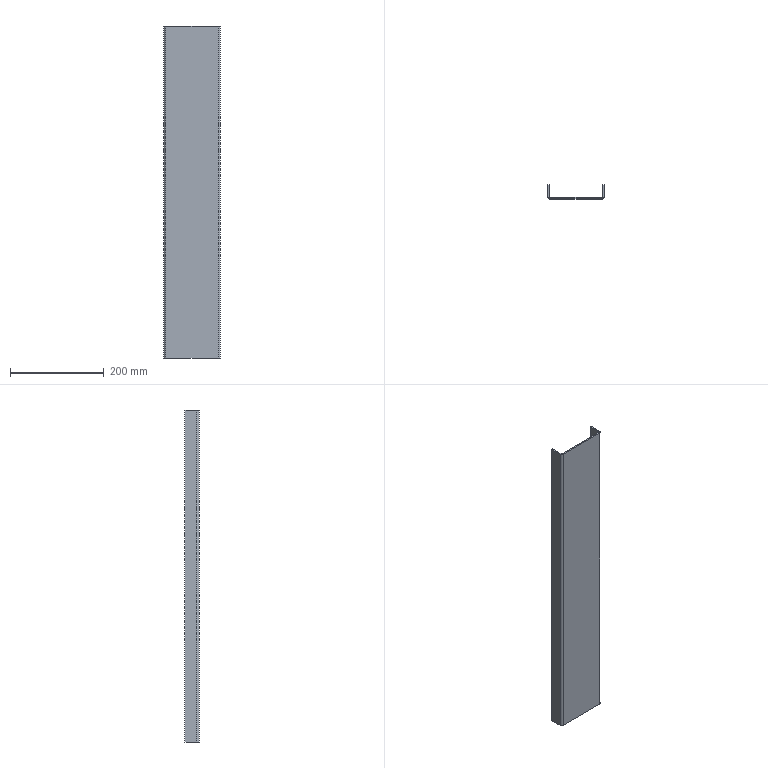Part | STEP file | Double-tube frame vertical brace SGN-1-05 | 1 solid | 22 faces | box 120 x 30 x 708 mm | volume 364106 mm3 | plane 18 | cylinder 4 | commonest cylinder face diameters 3 x2 9 x2
STEP:
#1=CARTESIAN_POINT('',(0.,0.,0.));
#2=DIRECTION('',(0.,0.,1.));
#3=DIRECTION('',(1.,0.,0.));
#4=AXIS2_PLACEMENT_3D('',#1,#2,#3);
#5=CARTESIAN_POINT('',(55.5,-6.24,708.));
#6=VERTEX_POINT('',#5);
#7=CARTESIAN_POINT('',(55.5,-3.24,708.));
#8=VERTEX_POINT('',#7);
#9=CARTESIAN_POINT('',(55.5,-6.24,708.));
#10=DIRECTION('',(0.,1.,0.));
#11=VECTOR('',#10,1.);
#12=LINE('',#9,#11);
#13=CARTESIAN_POINT('',(55.5,-6.24,708.));
#14=DIRECTION('',(0.,0.,1.));
#15=DIRECTION('',(1.,0.,0.));
#16=AXIS2_PLACEMENT_3D('',#13,#14,#15);
#17=PLANE('',#16);
#18=CARTESIAN_POINT('',(0.,0.));
#19=DIRECTION('',(0.,1.));
#20=VECTOR('',#19,1.);
#21=LINE('',#18,#20);
#22=(GEOMETRIC_REPRESENTATION_CONTEXT(2)PARAMETRIC_REPRESENTATION_CONTEXT()REPRESENTATION_CONTEXT('',''));
#23=DEFINITIONAL_REPRESENTATION('',(#21),#22);
#24=PCURVE('',#17,#23);
#25=CARTESIAN_POINT('',(57.,-1.74,708.));
#26=DIRECTION('',(0.,0.,1.));
#27=DIRECTION('',(1.,0.,0.));
#28=AXIS2_PLACEMENT_3D('',#25,#26,#27);
#29=PLANE('',#28);
#30=CARTESIAN_POINT('',(-1.5,-4.5));
#31=DIRECTION('',(0.,1.));
#32=VECTOR('',#31,1.);
#33=LINE('',#30,#32);
#34=(GEOMETRIC_REPRESENTATION_CONTEXT(2)PARAMETRIC_REPRESENTATION_CONTEXT()REPRESENTATION_CONTEXT('',''));
#35=DEFINITIONAL_REPRESENTATION('',(#33),#34);
#36=PCURVE('',#29,#35);
#37=SURFACE_CURVE('',#12,(#24,#36),.PCURVE_S1.);
#38=EDGE_CURVE('',#6,#8,#37,.T.);
#39=ORIENTED_EDGE('',*,*,#38,.F.);
#40=CARTESIAN_POINT('',(60.,-1.74,708.));
#41=VERTEX_POINT('',#40);
#42=CARTESIAN_POINT('',(55.5,-1.74,708.));
#43=DIRECTION('',(0.,0.,-1.));
#44=DIRECTION('',(1.,0.,0.));
#45=AXIS2_PLACEMENT_3D('',#42,#43,#44);
#46=CIRCLE('',#45,4.5);
#47=CARTESIAN_POINT('',(4.5,4.5));
#48=CARTESIAN_POINT('',(4.5,-3.294));
#49=CARTESIAN_POINT('',(-2.25,0.6029));
#50=CARTESIAN_POINT('',(-9.,4.5));
#51=CARTESIAN_POINT('',(-2.25,8.397));
#52=CARTESIAN_POINT('',(4.5,12.294));
#53=CARTESIAN_POINT('',(4.5,4.5));
#54=(BOUNDED_CURVE()B_SPLINE_CURVE(2,(#47,#48,#49,#50,#51,#52,#53),.UNSPECIFIED.,.T.,.F.)B_SPLINE_CURVE_WITH_KNOTS((1,2,2,2,2,1),(-2.094,0.,2.094,4.189,6.283,8.378),.UNSPECIFIED.)CURVE()GEOMETRIC_REPRESENTATION_ITEM()RATIONAL_B_SPLINE_CURVE((1.,0.5,1.,0.5,1.,0.5,1.))REPRESENTATION_ITEM(''));
#55=(GEOMETRIC_REPRESENTATION_CONTEXT(2)PARAMETRIC_REPRESENTATION_CONTEXT()REPRESENTATION_CONTEXT('',''));
#56=DEFINITIONAL_REPRESENTATION('',(#54),#55);
#57=PCURVE('',#17,#56);
#58=CARTESIAN_POINT('',(55.5,-1.74,708.));
#59=DIRECTION('',(0.,0.,-1.));
#60=DIRECTION('',(-1.,0.,0.));
#61=AXIS2_PLACEMENT_3D('',#58,#59,#60);
#62=CYLINDRICAL_SURFACE('',#61,4.5);
#63=CARTESIAN_POINT('',(3.142,0.));
#64=DIRECTION('',(1.,0.));
#65=VECTOR('',#64,1.);
#66=LINE('',#63,#65);
#67=(GEOMETRIC_REPRESENTATION_CONTEXT(2)PARAMETRIC_REPRESENTATION_CONTEXT()REPRESENTATION_CONTEXT('',''));
#68=DEFINITIONAL_REPRESENTATION('',(#66),#67);
#69=PCURVE('',#62,#68);
#70=SURFACE_CURVE('',#46,(#57,#69),.PCURVE_S1.);
#71=EDGE_CURVE('',#41,#6,#70,.T.);
#72=ORIENTED_EDGE('',*,*,#71,.F.);
#73=CARTESIAN_POINT('',(57.,-1.74,708.));
#74=VERTEX_POINT('',#73);
#75=CARTESIAN_POINT('',(57.,-1.74,708.));
#76=DIRECTION('',(1.,0.,0.));
#77=VECTOR('',#76,1.);
#78=LINE('',#75,#77);
#79=CARTESIAN_POINT('',(1.5,4.5));
#80=DIRECTION('',(1.,0.));
#81=VECTOR('',#80,1.);
#82=LINE('',#79,#81);
#83=(GEOMETRIC_REPRESENTATION_CONTEXT(2)PARAMETRIC_REPRESENTATION_CONTEXT()REPRESENTATION_CONTEXT('',''));
#84=DEFINITIONAL_REPRESENTATION('',(#82),#83);
#85=PCURVE('',#17,#84);
#86=CARTESIAN_POINT('',(-55.5,-1.74,708.));
#87=DIRECTION('',(0.,0.,1.));
#88=DIRECTION('',(1.,0.,0.));
#89=AXIS2_PLACEMENT_3D('',#86,#87,#88);
#90=PLANE('',#89);
#91=CARTESIAN_POINT('',(112.5,0.));
#92=DIRECTION('',(1.,0.));
#93=VECTOR('',#92,1.);
#94=LINE('',#91,#93);
#95=(GEOMETRIC_REPRESENTATION_CONTEXT(2)PARAMETRIC_REPRESENTATION_CONTEXT()REPRESENTATION_CONTEXT('',''));
#96=DEFINITIONAL_REPRESENTATION('',(#94),#95);
#97=PCURVE('',#90,#96);
#98=SURFACE_CURVE('',#78,(#85,#97),.PCURVE_S1.);
#99=EDGE_CURVE('',#74,#41,#98,.T.);
#100=ORIENTED_EDGE('',*,*,#99,.F.);
#101=CARTESIAN_POINT('',(55.5,-1.74,708.));
#102=DIRECTION('',(0.,0.,-1.));
#103=DIRECTION('',(1.,0.,0.));
#104=AXIS2_PLACEMENT_3D('',#101,#102,#103);
#105=CIRCLE('',#104,1.5);
#106=CARTESIAN_POINT('',(1.5,4.5));
#107=CARTESIAN_POINT('',(1.5,1.902));
#108=CARTESIAN_POINT('',(-0.75,3.201));
#109=CARTESIAN_POINT('',(-3.,4.5));
#110=CARTESIAN_POINT('',(-0.75,5.799));
#111=CARTESIAN_POINT('',(1.5,7.098));
#112=CARTESIAN_POINT('',(1.5,4.5));
#113=(BOUNDED_CURVE()B_SPLINE_CURVE(2,(#106,#107,#108,#109,#110,#111,#112),.UNSPECIFIED.,.T.,.F.)B_SPLINE_CURVE_WITH_KNOTS((1,2,2,2,2,1),(-2.094,0.,2.094,4.189,6.283,8.378),.UNSPECIFIED.)CURVE()GEOMETRIC_REPRESENTATION_ITEM()RATIONAL_B_SPLINE_CURVE((1.,0.5,1.,0.5,1.,0.5,1.))REPRESENTATION_ITEM(''));
#114=(GEOMETRIC_REPRESENTATION_CONTEXT(2)PARAMETRIC_REPRESENTATION_CONTEXT()REPRESENTATION_CONTEXT('',''));
#115=DEFINITIONAL_REPRESENTATION('',(#113),#114);
#116=PCURVE('',#17,#115);
#117=CARTESIAN_POINT('',(55.5,-1.74,708.));
#118=DIRECTION('',(0.,0.,-1.));
#119=DIRECTION('',(-1.,0.,0.));
#120=AXIS2_PLACEMENT_3D('',#117,#118,#119);
#121=CYLINDRICAL_SURFACE('',#120,1.5);
#122=CARTESIAN_POINT('',(3.142,0.));
#123=DIRECTION('',(1.,0.));
#124=VECTOR('',#123,1.);
#125=LINE('',#122,#124);
#126=(GEOMETRIC_REPRESENTATION_CONTEXT(2)PARAMETRIC_REPRESENTATION_CONTEXT()REPRESENTATION_CONTEXT('',''));
#127=DEFINITIONAL_REPRESENTATION('',(#125),#126);
#128=PCURVE('',#121,#127);
#129=SURFACE_CURVE('',#105,(#116,#128),.PCURVE_S1.);
#130=EDGE_CURVE('',#74,#8,#129,.T.);
#131=ORIENTED_EDGE('',*,*,#130,.T.);
#132=EDGE_LOOP('',(#39,#72,#100,#131));
#133=FACE_BOUND('',#132,.T.);
#134=ADVANCED_FACE('',(#133),#17,.T.);
#135=CARTESIAN_POINT('',(-55.5,-6.24,708.));
#136=VERTEX_POINT('',#135);
#137=CARTESIAN_POINT('',(-60.,-6.24,708.));
#138=DIRECTION('',(-1.,0.,0.));
#139=VECTOR('',#138,1.);
#140=LINE('',#137,#139);
#141=CARTESIAN_POINT('',(-117.,-4.5));
#142=DIRECTION('',(-1.,0.));
#143=VECTOR('',#142,1.);
#144=LINE('',#141,#143);
#145=(GEOMETRIC_REPRESENTATION_CONTEXT(2)PARAMETRIC_REPRESENTATION_CONTEXT()REPRESENTATION_CONTEXT('',''));
#146=DEFINITIONAL_REPRESENTATION('',(#144),#145);
#147=PCURVE('',#29,#146);
#148=CARTESIAN_POINT('',(-60.,-6.24,708.));
#149=DIRECTION('',(0.,-1.,0.));
#150=DIRECTION('',(0.,0.,-1.));
#151=AXIS2_PLACEMENT_3D('',#148,#149,#150);
#152=PLANE('',#151);
#153=CARTESIAN_POINT('',(0.,0.));
#154=DIRECTION('',(0.,-1.));
#155=VECTOR('',#154,1.);
#156=LINE('',#153,#155);
#157=(GEOMETRIC_REPRESENTATION_CONTEXT(2)PARAMETRIC_REPRESENTATION_CONTEXT()REPRESENTATION_CONTEXT('',''));
#158=DEFINITIONAL_REPRESENTATION('',(#156),#157);
#159=PCURVE('',#152,#158);
#160=SURFACE_CURVE('',#140,(#147,#159),.PCURVE_S1.);
#161=EDGE_CURVE('',#6,#136,#160,.T.);
#162=ORIENTED_EDGE('',*,*,#161,.F.);
#163=ORIENTED_EDGE('',*,*,#38,.T.);
#164=CARTESIAN_POINT('',(-55.5,-3.24,708.));
#165=VERTEX_POINT('',#164);
#166=CARTESIAN_POINT('',(-60.,-3.24,708.));
#167=DIRECTION('',(-1.,0.,0.));
#168=VECTOR('',#167,1.);
#169=LINE('',#166,#168);
#170=CARTESIAN_POINT('',(-117.,-1.5));
#171=DIRECTION('',(-1.,0.));
#172=VECTOR('',#171,1.);
#173=LINE('',#170,#172);
#174=(GEOMETRIC_REPRESENTATION_CONTEXT(2)PARAMETRIC_REPRESENTATION_CONTEXT()REPRESENTATION_CONTEXT('',''));
#175=DEFINITIONAL_REPRESENTATION('',(#173),#174);
#176=PCURVE('',#29,#175);
#177=CARTESIAN_POINT('',(-60.,-3.24,708.));
#178=DIRECTION('',(0.,-1.,0.));
#179=DIRECTION('',(0.,0.,-1.));
#180=AXIS2_PLACEMENT_3D('',#177,#178,#179);
#181=PLANE('',#180);
#182=CARTESIAN_POINT('',(0.,0.));
#183=DIRECTION('',(0.,-1.));
#184=VECTOR('',#183,1.);
#185=LINE('',#182,#184);
#186=(GEOMETRIC_REPRESENTATION_CONTEXT(2)PARAMETRIC_REPRESENTATION_CONTEXT()REPRESENTATION_CONTEXT('',''));
#187=DEFINITIONAL_REPRESENTATION('',(#185),#186);
#188=PCURVE('',#181,#187);
#189=SURFACE_CURVE('',#169,(#176,#188),.PCURVE_S1.);
#190=EDGE_CURVE('',#8,#165,#189,.T.);
#191=ORIENTED_EDGE('',*,*,#190,.T.);
#192=CARTESIAN_POINT('',(-55.5,-3.24,708.));
#193=DIRECTION('',(0.,-1.,0.));
#194=VECTOR('',#193,1.);
#195=LINE('',#192,#194);
#196=CARTESIAN_POINT('',(-112.5,-1.5));
#197=DIRECTION('',(0.,-1.));
#198=VECTOR('',#197,1.);
#199=LINE('',#196,#198);
#200=(GEOMETRIC_REPRESENTATION_CONTEXT(2)PARAMETRIC_REPRESENTATION_CONTEXT()REPRESENTATION_CONTEXT('',''));
#201=DEFINITIONAL_REPRESENTATION('',(#199),#200);
#202=PCURVE('',#29,#201);
#203=CARTESIAN_POINT('',(-60.,-1.74,708.));
#204=DIRECTION('',(0.,0.,1.));
#205=DIRECTION('',(1.,0.,0.));
#206=AXIS2_PLACEMENT_3D('',#203,#204,#205);
#207=PLANE('',#206);
#208=CARTESIAN_POINT('',(4.5,-1.5));
#209=DIRECTION('',(0.,-1.));
#210=VECTOR('',#209,1.);
#211=LINE('',#208,#210);
#212=(GEOMETRIC_REPRESENTATION_CONTEXT(2)PARAMETRIC_REPRESENTATION_CONTEXT()REPRESENTATION_CONTEXT('',''));
#213=DEFINITIONAL_REPRESENTATION('',(#211),#212);
#214=PCURVE('',#207,#213);
#215=SURFACE_CURVE('',#195,(#202,#214),.PCURVE_S1.);
#216=EDGE_CURVE('',#165,#136,#215,.T.);
#217=ORIENTED_EDGE('',*,*,#216,.T.);
#218=EDGE_LOOP('',(#162,#163,#191,#217));
#219=FACE_BOUND('',#218,.T.);
#220=ADVANCED_FACE('',(#219),#29,.T.);
#221=CARTESIAN_POINT('',(60.,-1.74,0.));
#222=VERTEX_POINT('',#221);
#223=CARTESIAN_POINT('',(57.,-1.74,0.));
#224=VERTEX_POINT('',#223);
#225=CARTESIAN_POINT('',(60.,-1.74,0.));
#226=DIRECTION('',(-1.,0.,0.));
#227=VECTOR('',#226,1.);
#228=LINE('',#225,#227);
#229=CARTESIAN_POINT('',(60.,-1.74,0.));
#230=DIRECTION('',(0.,0.,-1.));
#231=DIRECTION('',(-1.,0.,0.));
#232=AXIS2_PLACEMENT_3D('',#229,#230,#231);
#233=PLANE('',#232);
#234=CARTESIAN_POINT('',(0.,0.));
#235=DIRECTION('',(1.,0.));
#236=VECTOR('',#235,1.);
#237=LINE('',#234,#236);
#238=(GEOMETRIC_REPRESENTATION_CONTEXT(2)PARAMETRIC_REPRESENTATION_CONTEXT()REPRESENTATION_CONTEXT('',''));
#239=DEFINITIONAL_REPRESENTATION('',(#237),#238);
#240=PCURVE('',#233,#239);
#241=CARTESIAN_POINT('',(55.5,-3.24,0.));
#242=DIRECTION('',(0.,0.,-1.));
#243=DIRECTION('',(-1.,0.,0.));
#244=AXIS2_PLACEMENT_3D('',#241,#242,#243);
#245=PLANE('',#244);
#246=CARTESIAN_POINT('',(-4.5,1.5));
#247=DIRECTION('',(1.,0.));
#248=VECTOR('',#247,1.);
#249=LINE('',#246,#248);
#250=(GEOMETRIC_REPRESENTATION_CONTEXT(2)PARAMETRIC_REPRESENTATION_CONTEXT()REPRESENTATION_CONTEXT('',''));
#251=DEFINITIONAL_REPRESENTATION('',(#249),#250);
#252=PCURVE('',#245,#251);
#253=SURFACE_CURVE('',#228,(#240,#252),.PCURVE_S1.);
#254=EDGE_CURVE('',#222,#224,#253,.T.);
#255=ORIENTED_EDGE('',*,*,#254,.F.);
#256=CARTESIAN_POINT('',(55.5,-6.24,0.));
#257=VERTEX_POINT('',#256);
#258=CARTESIAN_POINT('',(55.5,-1.74,0.));
#259=DIRECTION('',(0.,0.,-1.));
#260=DIRECTION('',(1.,0.,0.));
#261=AXIS2_PLACEMENT_3D('',#258,#259,#260);
#262=CIRCLE('',#261,4.5);
#263=CARTESIAN_POINT('',(4.5,0.));
#264=DIRECTION('',(-1.,0.));
#265=AXIS2_PLACEMENT_2D('',#263,#264);
#266=CIRCLE('',#265,4.5);
#267=(GEOMETRIC_REPRESENTATION_CONTEXT(2)PARAMETRIC_REPRESENTATION_CONTEXT()REPRESENTATION_CONTEXT('',''));
#268=DEFINITIONAL_REPRESENTATION('',(#266),#267);
#269=PCURVE('',#233,#268);
#270=CARTESIAN_POINT('',(3.142,708.));
#271=DIRECTION('',(1.,0.));
#272=VECTOR('',#271,1.);
#273=LINE('',#270,#272);
#274=(GEOMETRIC_REPRESENTATION_CONTEXT(2)PARAMETRIC_REPRESENTATION_CONTEXT()REPRESENTATION_CONTEXT('',''));
#275=DEFINITIONAL_REPRESENTATION('',(#273),#274);
#276=PCURVE('',#62,#275);
#277=SURFACE_CURVE('',#262,(#269,#276),.PCURVE_S1.);
#278=EDGE_CURVE('',#222,#257,#277,.T.);
#279=ORIENTED_EDGE('',*,*,#278,.T.);
#280=CARTESIAN_POINT('',(55.5,-3.24,0.));
#281=VERTEX_POINT('',#280);
#282=CARTESIAN_POINT('',(55.5,-3.24,0.));
#283=DIRECTION('',(0.,-1.,0.));
#284=VECTOR('',#283,1.);
#285=LINE('',#282,#284);
#286=CARTESIAN_POINT('',(4.5,-1.5));
#287=DIRECTION('',(0.,-1.));
#288=VECTOR('',#287,1.);
#289=LINE('',#286,#288);
#290=(GEOMETRIC_REPRESENTATION_CONTEXT(2)PARAMETRIC_REPRESENTATION_CONTEXT()REPRESENTATION_CONTEXT('',''));
#291=DEFINITIONAL_REPRESENTATION('',(#289),#290);
#292=PCURVE('',#233,#291);
#293=CARTESIAN_POINT('',(-57.,-1.74,0.));
#294=DIRECTION('',(0.,0.,-1.));
#295=DIRECTION('',(-1.,0.,0.));
#296=AXIS2_PLACEMENT_3D('',#293,#294,#295);
#297=PLANE('',#296);
#298=CARTESIAN_POINT('',(-112.5,-1.5));
#299=DIRECTION('',(0.,-1.));
#300=VECTOR('',#299,1.);
#301=LINE('',#298,#300);
#302=(GEOMETRIC_REPRESENTATION_CONTEXT(2)PARAMETRIC_REPRESENTATION_CONTEXT()REPRESENTATION_CONTEXT('',''));
#303=DEFINITIONAL_REPRESENTATION('',(#301),#302);
#304=PCURVE('',#297,#303);
#305=SURFACE_CURVE('',#285,(#292,#304),.PCURVE_S1.);
#306=EDGE_CURVE('',#281,#257,#305,.T.);
#307=ORIENTED_EDGE('',*,*,#306,.F.);
#308=CARTESIAN_POINT('',(55.5,-1.74,0.));
#309=DIRECTION('',(0.,0.,-1.));
#310=DIRECTION('',(1.,0.,0.));
#311=AXIS2_PLACEMENT_3D('',#308,#309,#310);
#312=CIRCLE('',#311,1.5);
#313=CARTESIAN_POINT('',(4.5,0.));
#314=DIRECTION('',(-1.,0.));
#315=AXIS2_PLACEMENT_2D('',#313,#314);
#316=CIRCLE('',#315,1.5);
#317=(GEOMETRIC_REPRESENTATION_CONTEXT(2)PARAMETRIC_REPRESENTATION_CONTEXT()REPRESENTATION_CONTEXT('',''));
#318=DEFINITIONAL_REPRESENTATION('',(#316),#317);
#319=PCURVE('',#233,#318);
#320=CARTESIAN_POINT('',(3.142,708.));
#321=DIRECTION('',(1.,0.));
#322=VECTOR('',#321,1.);
#323=LINE('',#320,#322);
#324=(GEOMETRIC_REPRESENTATION_CONTEXT(2)PARAMETRIC_REPRESENTATION_CONTEXT()REPRESENTATION_CONTEXT('',''));
#325=DEFINITIONAL_REPRESENTATION('',(#323),#324);
#326=PCURVE('',#121,#325);
#327=SURFACE_CURVE('',#312,(#319,#326),.PCURVE_S1.);
#328=EDGE_CURVE('',#224,#281,#327,.T.);
#329=ORIENTED_EDGE('',*,*,#328,.F.);
#330=EDGE_LOOP('',(#255,#279,#307,#329));
#331=FACE_BOUND('',#330,.T.);
#332=ADVANCED_FACE('',(#331),#233,.T.);
#333=CARTESIAN_POINT('',(60.,23.76,0.));
#334=VERTEX_POINT('',#333);
#335=CARTESIAN_POINT('',(60.,-6.24,0.));
#336=DIRECTION('',(0.,-1.,0.));
#337=VECTOR('',#336,1.);
#338=LINE('',#335,#337);
#339=CARTESIAN_POINT('',(-4.5,-3.));
#340=DIRECTION('',(0.,-1.));
#341=VECTOR('',#340,1.);
#342=LINE('',#339,#341);
#343=(GEOMETRIC_REPRESENTATION_CONTEXT(2)PARAMETRIC_REPRESENTATION_CONTEXT()REPRESENTATION_CONTEXT('',''));
#344=DEFINITIONAL_REPRESENTATION('',(#342),#343);
#345=PCURVE('',#245,#344);
#346=CARTESIAN_POINT('',(60.,-6.24,708.));
#347=DIRECTION('',(1.,0.,0.));
#348=DIRECTION('',(0.,0.,-1.));
#349=AXIS2_PLACEMENT_3D('',#346,#347,#348);
#350=PLANE('',#349);
#351=CARTESIAN_POINT('',(708.,0.));
#352=DIRECTION('',(0.,-1.));
#353=VECTOR('',#352,1.);
#354=LINE('',#351,#353);
#355=(GEOMETRIC_REPRESENTATION_CONTEXT(2)PARAMETRIC_REPRESENTATION_CONTEXT()REPRESENTATION_CONTEXT('',''));
#356=DEFINITIONAL_REPRESENTATION('',(#354),#355);
#357=PCURVE('',#350,#356);
#358=SURFACE_CURVE('',#338,(#345,#357),.PCURVE_S1.);
#359=EDGE_CURVE('',#334,#222,#358,.T.);
#360=ORIENTED_EDGE('',*,*,#359,.T.);
#361=ORIENTED_EDGE('',*,*,#254,.T.);
#362=CARTESIAN_POINT('',(57.,23.76,0.));
#363=VERTEX_POINT('',#362);
#364=CARTESIAN_POINT('',(57.,-6.24,0.));
#365=DIRECTION('',(0.,-1.,0.));
#366=VECTOR('',#365,1.);
#367=LINE('',#364,#366);
#368=CARTESIAN_POINT('',(-1.5,-3.));
#369=DIRECTION('',(0.,-1.));
#370=VECTOR('',#369,1.);
#371=LINE('',#368,#370);
#372=(GEOMETRIC_REPRESENTATION_CONTEXT(2)PARAMETRIC_REPRESENTATION_CONTEXT()REPRESENTATION_CONTEXT('',''));
#373=DEFINITIONAL_REPRESENTATION('',(#371),#372);
#374=PCURVE('',#245,#373);
#375=CARTESIAN_POINT('',(57.,-6.24,708.));
#376=DIRECTION('',(1.,0.,0.));
#377=DIRECTION('',(0.,0.,-1.));
#378=AXIS2_PLACEMENT_3D('',#375,#376,#377);
#379=PLANE('',#378);
#380=CARTESIAN_POINT('',(708.,0.));
#381=DIRECTION('',(0.,-1.));
#382=VECTOR('',#381,1.);
#383=LINE('',#380,#382);
#384=(GEOMETRIC_REPRESENTATION_CONTEXT(2)PARAMETRIC_REPRESENTATION_CONTEXT()REPRESENTATION_CONTEXT('',''));
#385=DEFINITIONAL_REPRESENTATION('',(#383),#384);
#386=PCURVE('',#379,#385);
#387=SURFACE_CURVE('',#367,(#374,#386),.PCURVE_S1.);
#388=EDGE_CURVE('',#363,#224,#387,.T.);
#389=ORIENTED_EDGE('',*,*,#388,.F.);
#390=CARTESIAN_POINT('',(57.,23.76,0.));
#391=DIRECTION('',(1.,0.,0.));
#392=VECTOR('',#391,1.);
#393=LINE('',#390,#392);
#394=CARTESIAN_POINT('',(-1.5,27.));
#395=DIRECTION('',(-1.,0.));
#396=VECTOR('',#395,1.);
#397=LINE('',#394,#396);
#398=(GEOMETRIC_REPRESENTATION_CONTEXT(2)PARAMETRIC_REPRESENTATION_CONTEXT()REPRESENTATION_CONTEXT('',''));
#399=DEFINITIONAL_REPRESENTATION('',(#397),#398);
#400=PCURVE('',#245,#399);
#401=CARTESIAN_POINT('',(57.,23.76,708.));
#402=DIRECTION('',(0.,1.,0.));
#403=DIRECTION('',(0.,0.,1.));
#404=AXIS2_PLACEMENT_3D('',#401,#402,#403);
#405=PLANE('',#404);
#406=CARTESIAN_POINT('',(-708.,0.));
#407=DIRECTION('',(0.,1.));
#408=VECTOR('',#407,1.);
#409=LINE('',#406,#408);
#410=(GEOMETRIC_REPRESENTATION_CONTEXT(2)PARAMETRIC_REPRESENTATION_CONTEXT()REPRESENTATION_CONTEXT('',''));
#411=DEFINITIONAL_REPRESENTATION('',(#409),#410);
#412=PCURVE('',#405,#411);
#413=SURFACE_CURVE('',#393,(#400,#412),.PCURVE_S1.);
#414=EDGE_CURVE('',#363,#334,#413,.T.);
#415=ORIENTED_EDGE('',*,*,#414,.T.);
#416=EDGE_LOOP('',(#360,#361,#389,#415));
#417=FACE_BOUND('',#416,.T.);
#418=ADVANCED_FACE('',(#417),#245,.T.);
#419=CARTESIAN_POINT('',(-60.,-1.74,708.));
#420=VERTEX_POINT('',#419);
#421=CARTESIAN_POINT('',(-57.,-1.74,708.));
#422=VERTEX_POINT('',#421);
#423=CARTESIAN_POINT('',(-60.,-1.74,708.));
#424=DIRECTION('',(1.,0.,0.));
#425=VECTOR('',#424,1.);
#426=LINE('',#423,#425);
#427=CARTESIAN_POINT('',(0.,0.));
#428=DIRECTION('',(1.,0.));
#429=VECTOR('',#428,1.);
#430=LINE('',#427,#429);
#431=(GEOMETRIC_REPRESENTATION_CONTEXT(2)PARAMETRIC_REPRESENTATION_CONTEXT()REPRESENTATION_CONTEXT('',''));
#432=DEFINITIONAL_REPRESENTATION('',(#430),#431);
#433=PCURVE('',#207,#432);
#434=CARTESIAN_POINT('',(-55.5,-3.24,708.));
#435=DIRECTION('',(0.,0.,1.));
#436=DIRECTION('',(1.,0.,0.));
#437=AXIS2_PLACEMENT_3D('',#434,#435,#436);
#438=PLANE('',#437);
#439=CARTESIAN_POINT('',(-4.5,1.5));
#440=DIRECTION('',(1.,0.));
#441=VECTOR('',#440,1.);
#442=LINE('',#439,#441);
#443=(GEOMETRIC_REPRESENTATION_CONTEXT(2)PARAMETRIC_REPRESENTATION_CONTEXT()REPRESENTATION_CONTEXT('',''));
#444=DEFINITIONAL_REPRESENTATION('',(#442),#443);
#445=PCURVE('',#438,#444);
#446=SURFACE_CURVE('',#426,(#433,#445),.PCURVE_S1.);
#447=EDGE_CURVE('',#420,#422,#446,.T.);
#448=ORIENTED_EDGE('',*,*,#447,.F.);
#449=CARTESIAN_POINT('',(-55.5,-1.74,708.));
#450=DIRECTION('',(0.,0.,-1.));
#451=DIRECTION('',(1.,0.,0.));
#452=AXIS2_PLACEMENT_3D('',#449,#450,#451);
#453=CIRCLE('',#452,4.5);
#454=CARTESIAN_POINT('',(9.,0.));
#455=CARTESIAN_POINT('',(9.,-7.794));
#456=CARTESIAN_POINT('',(2.25,-3.897));
#457=CARTESIAN_POINT('',(-4.5,0.));
#458=CARTESIAN_POINT('',(2.25,3.897));
#459=CARTESIAN_POINT('',(9.,7.794));
#460=CARTESIAN_POINT('',(9.,0.));
#461=(BOUNDED_CURVE()B_SPLINE_CURVE(2,(#454,#455,#456,#457,#458,#459,#460),.UNSPECIFIED.,.T.,.F.)B_SPLINE_CURVE_WITH_KNOTS((1,2,2,2,2,1),(-2.094,0.,2.094,4.189,6.283,8.378),.UNSPECIFIED.)CURVE()GEOMETRIC_REPRESENTATION_ITEM()RATIONAL_B_SPLINE_CURVE((1.,0.5,1.,0.5,1.,0.5,1.))REPRESENTATION_ITEM(''));
#462=(GEOMETRIC_REPRESENTATION_CONTEXT(2)PARAMETRIC_REPRESENTATION_CONTEXT()REPRESENTATION_CONTEXT('',''));
#463=DEFINITIONAL_REPRESENTATION('',(#461),#462);
#464=PCURVE('',#207,#463);
#465=CARTESIAN_POINT('',(-55.5,-1.74,708.));
#466=DIRECTION('',(0.,0.,-1.));
#467=DIRECTION('',(-1.,0.,0.));
#468=AXIS2_PLACEMENT_3D('',#465,#466,#467);
#469=CYLINDRICAL_SURFACE('',#468,4.5);
#470=CARTESIAN_POINT('',(3.142,0.));
#471=DIRECTION('',(1.,0.));
#472=VECTOR('',#471,1.);
#473=LINE('',#470,#472);
#474=(GEOMETRIC_REPRESENTATION_CONTEXT(2)PARAMETRIC_REPRESENTATION_CONTEXT()REPRESENTATION_CONTEXT('',''));
#475=DEFINITIONAL_REPRESENTATION('',(#473),#474);
#476=PCURVE('',#469,#475);
#477=SURFACE_CURVE('',#453,(#464,#476),.PCURVE_S1.);
#478=EDGE_CURVE('',#136,#420,#477,.T.);
#479=ORIENTED_EDGE('',*,*,#478,.F.);
#480=ORIENTED_EDGE('',*,*,#216,.F.);
#481=CARTESIAN_POINT('',(-55.5,-1.74,708.));
#482=DIRECTION('',(0.,0.,-1.));
#483=DIRECTION('',(1.,0.,0.));
#484=AXIS2_PLACEMENT_3D('',#481,#482,#483);
#485=CIRCLE('',#484,1.5);
#486=CARTESIAN_POINT('',(6.,0.));
#487=CARTESIAN_POINT('',(6.,-2.598));
#488=CARTESIAN_POINT('',(3.75,-1.299));
#489=CARTESIAN_POINT('',(1.5,0.));
#490=CARTESIAN_POINT('',(3.75,1.299));
#491=CARTESIAN_POINT('',(6.,2.598));
#492=CARTESIAN_POINT('',(6.,0.));
#493=(BOUNDED_CURVE()B_SPLINE_CURVE(2,(#486,#487,#488,#489,#490,#491,#492),.UNSPECIFIED.,.T.,.F.)B_SPLINE_CURVE_WITH_KNOTS((1,2,2,2,2,1),(-2.094,0.,2.094,4.189,6.283,8.378),.UNSPECIFIED.)CURVE()GEOMETRIC_REPRESENTATION_ITEM()RATIONAL_B_SPLINE_CURVE((1.,0.5,1.,0.5,1.,0.5,1.))REPRESENTATION_ITEM(''));
#494=(GEOMETRIC_REPRESENTATION_CONTEXT(2)PARAMETRIC_REPRESENTATION_CONTEXT()REPRESENTATION_CONTEXT('',''));
#495=DEFINITIONAL_REPRESENTATION('',(#493),#494);
#496=PCURVE('',#207,#495);
#497=CARTESIAN_POINT('',(-55.5,-1.74,708.));
#498=DIRECTION('',(0.,0.,-1.));
#499=DIRECTION('',(-1.,0.,0.));
#500=AXIS2_PLACEMENT_3D('',#497,#498,#499);
#501=CYLINDRICAL_SURFACE('',#500,1.5);
#502=CARTESIAN_POINT('',(3.142,0.));
#503=DIRECTION('',(1.,0.));
#504=VECTOR('',#503,1.);
#505=LINE('',#502,#504);
#506=(GEOMETRIC_REPRESENTATION_CONTEXT(2)PARAMETRIC_REPRESENTATION_CONTEXT()REPRESENTATION_CONTEXT('',''));
#507=DEFINITIONAL_REPRESENTATION('',(#505),#506);
#508=PCURVE('',#501,#507);
#509=SURFACE_CURVE('',#485,(#496,#508),.PCURVE_S1.);
#510=EDGE_CURVE('',#165,#422,#509,.T.);
#511=ORIENTED_EDGE('',*,*,#510,.T.);
#512=EDGE_LOOP('',(#448,#479,#480,#511));
#513=FACE_BOUND('',#512,.T.);
#514=ADVANCED_FACE('',(#513),#207,.T.);
#515=CARTESIAN_POINT('',(-60.,23.76,708.));
#516=VERTEX_POINT('',#515);
#517=CARTESIAN_POINT('',(-60.,-6.24,708.));
#518=DIRECTION('',(0.,1.,0.));
#519=VECTOR('',#518,1.);
#520=LINE('',#517,#519);
#521=CARTESIAN_POINT('',(-4.5,-3.));
#522=DIRECTION('',(0.,1.));
#523=VECTOR('',#522,1.);
#524=LINE('',#521,#523);
#525=(GEOMETRIC_REPRESENTATION_CONTEXT(2)PARAMETRIC_REPRESENTATION_CONTEXT()REPRESENTATION_CONTEXT('',''));
#526=DEFINITIONAL_REPRESENTATION('',(#524),#525);
#527=PCURVE('',#438,#526);
#528=CARTESIAN_POINT('',(-60.,-6.24,708.));
#529=DIRECTION('',(-1.,0.,0.));
#530=DIRECTION('',(0.,0.,1.));
#531=AXIS2_PLACEMENT_3D('',#528,#529,#530);
#532=PLANE('',#531);
#533=CARTESIAN_POINT('',(0.,0.));
#534=DIRECTION('',(0.,1.));
#535=VECTOR('',#534,1.);
#536=LINE('',#533,#535);
#537=(GEOMETRIC_REPRESENTATION_CONTEXT(2)PARAMETRIC_REPRESENTATION_CONTEXT()REPRESENTATION_CONTEXT('',''));
#538=DEFINITIONAL_REPRESENTATION('',(#536),#537);
#539=PCURVE('',#532,#538);
#540=SURFACE_CURVE('',#520,(#527,#539),.PCURVE_S1.);
#541=EDGE_CURVE('',#420,#516,#540,.T.);
#542=ORIENTED_EDGE('',*,*,#541,.F.);
#543=ORIENTED_EDGE('',*,*,#447,.T.);
#544=CARTESIAN_POINT('',(-57.,23.76,708.));
#545=VERTEX_POINT('',#544);
#546=CARTESIAN_POINT('',(-57.,-6.24,708.));
#547=DIRECTION('',(0.,1.,0.));
#548=VECTOR('',#547,1.);
#549=LINE('',#546,#548);
#550=CARTESIAN_POINT('',(-1.5,-3.));
#551=DIRECTION('',(0.,1.));
#552=VECTOR('',#551,1.);
#553=LINE('',#550,#552);
#554=(GEOMETRIC_REPRESENTATION_CONTEXT(2)PARAMETRIC_REPRESENTATION_CONTEXT()REPRESENTATION_CONTEXT('',''));
#555=DEFINITIONAL_REPRESENTATION('',(#553),#554);
#556=PCURVE('',#438,#555);
#557=CARTESIAN_POINT('',(-57.,-6.24,708.));
#558=DIRECTION('',(-1.,0.,0.));
#559=DIRECTION('',(0.,0.,1.));
#560=AXIS2_PLACEMENT_3D('',#557,#558,#559);
#561=PLANE('',#560);
#562=CARTESIAN_POINT('',(0.,0.));
#563=DIRECTION('',(0.,1.));
#564=VECTOR('',#563,1.);
#565=LINE('',#562,#564);
#566=(GEOMETRIC_REPRESENTATION_CONTEXT(2)PARAMETRIC_REPRESENTATION_CONTEXT()REPRESENTATION_CONTEXT('',''));
#567=DEFINITIONAL_REPRESENTATION('',(#565),#566);
#568=PCURVE('',#561,#567);
#569=SURFACE_CURVE('',#549,(#556,#568),.PCURVE_S1.);
#570=EDGE_CURVE('',#422,#545,#569,.T.);
#571=ORIENTED_EDGE('',*,*,#570,.T.);
#572=CARTESIAN_POINT('',(-60.,23.76,708.));
#573=DIRECTION('',(1.,0.,0.));
#574=VECTOR('',#573,1.);
#575=LINE('',#572,#574);
#576=CARTESIAN_POINT('',(-4.5,27.));
#577=DIRECTION('',(1.,0.));
#578=VECTOR('',#577,1.);
#579=LINE('',#576,#578);
#580=(GEOMETRIC_REPRESENTATION_CONTEXT(2)PARAMETRIC_REPRESENTATION_CONTEXT()REPRESENTATION_CONTEXT('',''));
#581=DEFINITIONAL_REPRESENTATION('',(#579),#580);
#582=PCURVE('',#438,#581);
#583=CARTESIAN_POINT('',(-60.,23.76,708.));
#584=DIRECTION('',(0.,1.,0.));
#585=DIRECTION('',(0.,0.,1.));
#586=AXIS2_PLACEMENT_3D('',#583,#584,#585);
#587=PLANE('',#586);
#588=CARTESIAN_POINT('',(0.,0.));
#589=DIRECTION('',(0.,1.));
#590=VECTOR('',#589,1.);
#591=LINE('',#588,#590);
#592=(GEOMETRIC_REPRESENTATION_CONTEXT(2)PARAMETRIC_REPRESENTATION_CONTEXT()REPRESENTATION_CONTEXT('',''));
#593=DEFINITIONAL_REPRESENTATION('',(#591),#592);
#594=PCURVE('',#587,#593);
#595=SURFACE_CURVE('',#575,(#582,#594),.PCURVE_S1.);
#596=EDGE_CURVE('',#516,#545,#595,.T.);
#597=ORIENTED_EDGE('',*,*,#596,.F.);
#598=EDGE_LOOP('',(#542,#543,#571,#597));
#599=FACE_BOUND('',#598,.T.);
#600=ADVANCED_FACE('',(#599),#438,.T.);
#601=CARTESIAN_POINT('',(-55.5,-6.24,0.));
#602=VERTEX_POINT('',#601);
#603=CARTESIAN_POINT('',(-55.5,-3.24,0.));
#604=VERTEX_POINT('',#603);
#605=CARTESIAN_POINT('',(-55.5,-6.24,0.));
#606=DIRECTION('',(0.,1.,0.));
#607=VECTOR('',#606,1.);
#608=LINE('',#605,#607);
#609=CARTESIAN_POINT('',(-55.5,-6.24,0.));
#610=DIRECTION('',(0.,0.,-1.));
#611=DIRECTION('',(-1.,0.,0.));
#612=AXIS2_PLACEMENT_3D('',#609,#610,#611);
#613=PLANE('',#612);
#614=CARTESIAN_POINT('',(0.,0.));
#615=DIRECTION('',(0.,1.));
#616=VECTOR('',#615,1.);
#617=LINE('',#614,#616);
#618=(GEOMETRIC_REPRESENTATION_CONTEXT(2)PARAMETRIC_REPRESENTATION_CONTEXT()REPRESENTATION_CONTEXT('',''));
#619=DEFINITIONAL_REPRESENTATION('',(#617),#618);
#620=PCURVE('',#613,#619);
#621=CARTESIAN_POINT('',(-1.5,-4.5));
#622=DIRECTION('',(0.,1.));
#623=VECTOR('',#622,1.);
#624=LINE('',#621,#623);
#625=(GEOMETRIC_REPRESENTATION_CONTEXT(2)PARAMETRIC_REPRESENTATION_CONTEXT()REPRESENTATION_CONTEXT('',''));
#626=DEFINITIONAL_REPRESENTATION('',(#624),#625);
#627=PCURVE('',#297,#626);
#628=SURFACE_CURVE('',#608,(#620,#627),.PCURVE_S1.);
#629=EDGE_CURVE('',#602,#604,#628,.T.);
#630=ORIENTED_EDGE('',*,*,#629,.F.);
#631=CARTESIAN_POINT('',(-60.,-1.74,0.));
#632=VERTEX_POINT('',#631);
#633=CARTESIAN_POINT('',(-55.5,-1.74,0.));
#634=DIRECTION('',(0.,0.,-1.));
#635=DIRECTION('',(1.,0.,0.));
#636=AXIS2_PLACEMENT_3D('',#633,#634,#635);
#637=CIRCLE('',#636,4.5);
#638=CARTESIAN_POINT('',(0.,4.5));
#639=DIRECTION('',(-1.,0.));
#640=AXIS2_PLACEMENT_2D('',#638,#639);
#641=CIRCLE('',#640,4.5);
#642=(GEOMETRIC_REPRESENTATION_CONTEXT(2)PARAMETRIC_REPRESENTATION_CONTEXT()REPRESENTATION_CONTEXT('',''));
#643=DEFINITIONAL_REPRESENTATION('',(#641),#642);
#644=PCURVE('',#613,#643);
#645=CARTESIAN_POINT('',(3.142,708.));
#646=DIRECTION('',(1.,0.));
#647=VECTOR('',#646,1.);
#648=LINE('',#645,#647);
#649=(GEOMETRIC_REPRESENTATION_CONTEXT(2)PARAMETRIC_REPRESENTATION_CONTEXT()REPRESENTATION_CONTEXT('',''));
#650=DEFINITIONAL_REPRESENTATION('',(#648),#649);
#651=PCURVE('',#469,#650);
#652=SURFACE_CURVE('',#637,(#644,#651),.PCURVE_S1.);
#653=EDGE_CURVE('',#602,#632,#652,.T.);
#654=ORIENTED_EDGE('',*,*,#653,.T.);
#655=CARTESIAN_POINT('',(-57.,-1.74,0.));
#656=VERTEX_POINT('',#655);
#657=CARTESIAN_POINT('',(-57.,-1.74,0.));
#658=DIRECTION('',(-1.,0.,0.));
#659=VECTOR('',#658,1.);
#660=LINE('',#657,#659);
#661=CARTESIAN_POINT('',(1.5,4.5));
#662=DIRECTION('',(1.,0.));
#663=VECTOR('',#662,1.);
#664=LINE('',#661,#663);
#665=(GEOMETRIC_REPRESENTATION_CONTEXT(2)PARAMETRIC_REPRESENTATION_CONTEXT()REPRESENTATION_CONTEXT('',''));
#666=DEFINITIONAL_REPRESENTATION('',(#664),#665);
#667=PCURVE('',#613,#666);
#668=CARTESIAN_POINT('',(-55.5,-1.74,0.));
#669=DIRECTION('',(0.,0.,1.));
#670=DIRECTION('',(1.,0.,0.));
#671=AXIS2_PLACEMENT_3D('',#668,#669,#670);
#672=PLANE('',#671);
#673=CARTESIAN_POINT('',(-1.5,0.));
#674=DIRECTION('',(-1.,0.));
#675=VECTOR('',#674,1.);
#676=LINE('',#673,#675);
#677=(GEOMETRIC_REPRESENTATION_CONTEXT(2)PARAMETRIC_REPRESENTATION_CONTEXT()REPRESENTATION_CONTEXT('',''));
#678=DEFINITIONAL_REPRESENTATION('',(#676),#677);
#679=PCURVE('',#672,#678);
#680=SURFACE_CURVE('',#660,(#667,#679),.PCURVE_S1.);
#681=EDGE_CURVE('',#656,#632,#680,.T.);
#682=ORIENTED_EDGE('',*,*,#681,.F.);
#683=CARTESIAN_POINT('',(-55.5,-1.74,0.));
#684=DIRECTION('',(0.,0.,-1.));
#685=DIRECTION('',(1.,0.,0.));
#686=AXIS2_PLACEMENT_3D('',#683,#684,#685);
#687=CIRCLE('',#686,1.5);
#688=CARTESIAN_POINT('',(0.,4.5));
#689=DIRECTION('',(-1.,0.));
#690=AXIS2_PLACEMENT_2D('',#688,#689);
#691=CIRCLE('',#690,1.5);
#692=(GEOMETRIC_REPRESENTATION_CONTEXT(2)PARAMETRIC_REPRESENTATION_CONTEXT()REPRESENTATION_CONTEXT('',''));
#693=DEFINITIONAL_REPRESENTATION('',(#691),#692);
#694=PCURVE('',#613,#693);
#695=CARTESIAN_POINT('',(3.142,708.));
#696=DIRECTION('',(1.,0.));
#697=VECTOR('',#696,1.);
#698=LINE('',#695,#697);
#699=(GEOMETRIC_REPRESENTATION_CONTEXT(2)PARAMETRIC_REPRESENTATION_CONTEXT()REPRESENTATION_CONTEXT('',''));
#700=DEFINITIONAL_REPRESENTATION('',(#698),#699);
#701=PCURVE('',#501,#700);
#702=SURFACE_CURVE('',#687,(#694,#701),.PCURVE_S1.);
#703=EDGE_CURVE('',#604,#656,#702,.T.);
#704=ORIENTED_EDGE('',*,*,#703,.F.);
#705=EDGE_LOOP('',(#630,#654,#682,#704));
#706=FACE_BOUND('',#705,.T.);
#707=ADVANCED_FACE('',(#706),#613,.T.);
#708=CARTESIAN_POINT('',(-60.,-6.24,0.));
#709=DIRECTION('',(-1.,0.,0.));
#710=VECTOR('',#709,1.);
#711=LINE('',#708,#710);
#712=CARTESIAN_POINT('',(3.,-4.5));
#713=DIRECTION('',(1.,0.));
#714=VECTOR('',#713,1.);
#715=LINE('',#712,#714);
#716=(GEOMETRIC_REPRESENTATION_CONTEXT(2)PARAMETRIC_REPRESENTATION_CONTEXT()REPRESENTATION_CONTEXT('',''));
#717=DEFINITIONAL_REPRESENTATION('',(#715),#716);
#718=PCURVE('',#297,#717);
#719=CARTESIAN_POINT('',(708.,0.));
#720=DIRECTION('',(0.,-1.));
#721=VECTOR('',#720,1.);
#722=LINE('',#719,#721);
#723=(GEOMETRIC_REPRESENTATION_CONTEXT(2)PARAMETRIC_REPRESENTATION_CONTEXT()REPRESENTATION_CONTEXT('',''));
#724=DEFINITIONAL_REPRESENTATION('',(#722),#723);
#725=PCURVE('',#152,#724);
#726=SURFACE_CURVE('',#711,(#718,#725),.PCURVE_S1.);
#727=EDGE_CURVE('',#257,#602,#726,.T.);
#728=ORIENTED_EDGE('',*,*,#727,.T.);
#729=ORIENTED_EDGE('',*,*,#629,.T.);
#730=CARTESIAN_POINT('',(-60.,-3.24,0.));
#731=DIRECTION('',(-1.,0.,0.));
#732=VECTOR('',#731,1.);
#733=LINE('',#730,#732);
#734=CARTESIAN_POINT('',(3.,-1.5));
#735=DIRECTION('',(1.,0.));
#736=VECTOR('',#735,1.);
#737=LINE('',#734,#736);
#738=(GEOMETRIC_REPRESENTATION_CONTEXT(2)PARAMETRIC_REPRESENTATION_CONTEXT()REPRESENTATION_CONTEXT('',''));
#739=DEFINITIONAL_REPRESENTATION('',(#737),#738);
#740=PCURVE('',#297,#739);
#741=CARTESIAN_POINT('',(708.,0.));
#742=DIRECTION('',(0.,-1.));
#743=VECTOR('',#742,1.);
#744=LINE('',#741,#743);
#745=(GEOMETRIC_REPRESENTATION_CONTEXT(2)PARAMETRIC_REPRESENTATION_CONTEXT()REPRESENTATION_CONTEXT('',''));
#746=DEFINITIONAL_REPRESENTATION('',(#744),#745);
#747=PCURVE('',#181,#746);
#748=SURFACE_CURVE('',#733,(#740,#747),.PCURVE_S1.);
#749=EDGE_CURVE('',#281,#604,#748,.T.);
#750=ORIENTED_EDGE('',*,*,#749,.F.);
#751=ORIENTED_EDGE('',*,*,#306,.T.);
#752=EDGE_LOOP('',(#728,#729,#750,#751));
#753=FACE_BOUND('',#752,.T.);
#754=ADVANCED_FACE('',(#753),#297,.T.);
#755=CARTESIAN_POINT('',(-57.,23.76,0.));
#756=VERTEX_POINT('',#755);
#757=CARTESIAN_POINT('',(-57.,-6.24,0.));
#758=DIRECTION('',(0.,1.,0.));
#759=VECTOR('',#758,1.);
#760=LINE('',#757,#759);
#761=CARTESIAN_POINT('',(-708.,0.));
#762=DIRECTION('',(0.,1.));
#763=VECTOR('',#762,1.);
#764=LINE('',#761,#763);
#765=(GEOMETRIC_REPRESENTATION_CONTEXT(2)PARAMETRIC_REPRESENTATION_CONTEXT()REPRESENTATION_CONTEXT('',''));
#766=DEFINITIONAL_REPRESENTATION('',(#764),#765);
#767=PCURVE('',#561,#766);
#768=CARTESIAN_POINT('',(-1.5,-4.5));
#769=DIRECTION('',(0.,1.));
#770=VECTOR('',#769,1.);
#771=LINE('',#768,#770);
#772=(GEOMETRIC_REPRESENTATION_CONTEXT(2)PARAMETRIC_REPRESENTATION_CONTEXT()REPRESENTATION_CONTEXT('',''));
#773=DEFINITIONAL_REPRESENTATION('',(#771),#772);
#774=PCURVE('',#672,#773);
#775=SURFACE_CURVE('',#760,(#767,#774),.PCURVE_S1.);
#776=EDGE_CURVE('',#656,#756,#775,.T.);
#777=ORIENTED_EDGE('',*,*,#776,.T.);
#778=CARTESIAN_POINT('',(-57.,23.76,708.));
#779=DIRECTION('',(0.,0.,-1.));
#780=VECTOR('',#779,1.);
#781=LINE('',#778,#780);
#782=CARTESIAN_POINT('',(0.,30.));
#783=DIRECTION('',(-1.,0.));
#784=VECTOR('',#783,1.);
#785=LINE('',#782,#784);
#786=(GEOMETRIC_REPRESENTATION_CONTEXT(2)PARAMETRIC_REPRESENTATION_CONTEXT()REPRESENTATION_CONTEXT('',''));
#787=DEFINITIONAL_REPRESENTATION('',(#785),#786);
#788=PCURVE('',#561,#787);
#789=CARTESIAN_POINT('',(0.,3.));
#790=DIRECTION('',(-1.,0.));
#791=VECTOR('',#790,1.);
#792=LINE('',#789,#791);
#793=(GEOMETRIC_REPRESENTATION_CONTEXT(2)PARAMETRIC_REPRESENTATION_CONTEXT()REPRESENTATION_CONTEXT('',''));
#794=DEFINITIONAL_REPRESENTATION('',(#792),#793);
#795=PCURVE('',#587,#794);
#796=SURFACE_CURVE('',#781,(#788,#795),.PCURVE_S1.);
#797=EDGE_CURVE('',#545,#756,#796,.T.);
#798=ORIENTED_EDGE('',*,*,#797,.F.);
#799=ORIENTED_EDGE('',*,*,#570,.F.);
#800=CARTESIAN_POINT('',(-57.,-1.74,708.));
#801=DIRECTION('',(0.,0.,-1.));
#802=VECTOR('',#801,1.);
#803=LINE('',#800,#802);
#804=CARTESIAN_POINT('',(0.,4.5));
#805=DIRECTION('',(-1.,0.));
#806=VECTOR('',#805,1.);
#807=LINE('',#804,#806);
#808=(GEOMETRIC_REPRESENTATION_CONTEXT(2)PARAMETRIC_REPRESENTATION_CONTEXT()REPRESENTATION_CONTEXT('',''));
#809=DEFINITIONAL_REPRESENTATION('',(#807),#808);
#810=PCURVE('',#561,#809);
#811=CARTESIAN_POINT('',(6.283,0.));
#812=DIRECTION('',(0.,1.));
#813=VECTOR('',#812,1.);
#814=LINE('',#811,#813);
#815=(GEOMETRIC_REPRESENTATION_CONTEXT(2)PARAMETRIC_REPRESENTATION_CONTEXT()REPRESENTATION_CONTEXT('',''));
#816=DEFINITIONAL_REPRESENTATION('',(#814),#815);
#817=PCURVE('',#501,#816);
#818=SURFACE_CURVE('',#803,(#810,#817),.PCURVE_S1.);
#819=EDGE_CURVE('',#422,#656,#818,.T.);
#820=ORIENTED_EDGE('',*,*,#819,.T.);
#821=EDGE_LOOP('',(#777,#798,#799,#820));
#822=FACE_BOUND('',#821,.T.);
#823=ADVANCED_FACE('',(#822),#561,.F.);
#824=CARTESIAN_POINT('',(-60.,23.76,0.));
#825=VERTEX_POINT('',#824);
#826=CARTESIAN_POINT('',(-60.,23.76,0.));
#827=DIRECTION('',(1.,0.,0.));
#828=VECTOR('',#827,1.);
#829=LINE('',#826,#828);
#830=CARTESIAN_POINT('',(-708.,0.));
#831=DIRECTION('',(0.,1.));
#832=VECTOR('',#831,1.);
#833=LINE('',#830,#832);
#834=(GEOMETRIC_REPRESENTATION_CONTEXT(2)PARAMETRIC_REPRESENTATION_CONTEXT()REPRESENTATION_CONTEXT('',''));
#835=DEFINITIONAL_REPRESENTATION('',(#833),#834);
#836=PCURVE('',#587,#835);
#837=CARTESIAN_POINT('',(-4.5,25.5));
#838=DIRECTION('',(1.,0.));
#839=VECTOR('',#838,1.);
#840=LINE('',#837,#839);
#841=(GEOMETRIC_REPRESENTATION_CONTEXT(2)PARAMETRIC_REPRESENTATION_CONTEXT()REPRESENTATION_CONTEXT('',''));
#842=DEFINITIONAL_REPRESENTATION('',(#840),#841);
#843=PCURVE('',#672,#842);
#844=SURFACE_CURVE('',#829,(#836,#843),.PCURVE_S1.);
#845=EDGE_CURVE('',#825,#756,#844,.T.);
#846=ORIENTED_EDGE('',*,*,#845,.F.);
#847=CARTESIAN_POINT('',(-60.,23.76,708.));
#848=DIRECTION('',(0.,0.,-1.));
#849=VECTOR('',#848,1.);
#850=LINE('',#847,#849);
#851=CARTESIAN_POINT('',(0.,0.));
#852=DIRECTION('',(-1.,0.));
#853=VECTOR('',#852,1.);
#854=LINE('',#851,#853);
#855=(GEOMETRIC_REPRESENTATION_CONTEXT(2)PARAMETRIC_REPRESENTATION_CONTEXT()REPRESENTATION_CONTEXT('',''));
#856=DEFINITIONAL_REPRESENTATION('',(#854),#855);
#857=PCURVE('',#587,#856);
#858=CARTESIAN_POINT('',(0.,30.));
#859=DIRECTION('',(-1.,0.));
#860=VECTOR('',#859,1.);
#861=LINE('',#858,#860);
#862=(GEOMETRIC_REPRESENTATION_CONTEXT(2)PARAMETRIC_REPRESENTATION_CONTEXT()REPRESENTATION_CONTEXT('',''));
#863=DEFINITIONAL_REPRESENTATION('',(#861),#862);
#864=PCURVE('',#532,#863);
#865=SURFACE_CURVE('',#850,(#857,#864),.PCURVE_S1.);
#866=EDGE_CURVE('',#516,#825,#865,.T.);
#867=ORIENTED_EDGE('',*,*,#866,.F.);
#868=ORIENTED_EDGE('',*,*,#596,.T.);
#869=ORIENTED_EDGE('',*,*,#797,.T.);
#870=EDGE_LOOP('',(#846,#867,#868,#869));
#871=FACE_BOUND('',#870,.T.);
#872=ADVANCED_FACE('',(#871),#587,.T.);
#873=CARTESIAN_POINT('',(-60.,-6.24,0.));
#874=DIRECTION('',(0.,1.,0.));
#875=VECTOR('',#874,1.);
#876=LINE('',#873,#875);
#877=CARTESIAN_POINT('',(-708.,0.));
#878=DIRECTION('',(0.,1.));
#879=VECTOR('',#878,1.);
#880=LINE('',#877,#879);
#881=(GEOMETRIC_REPRESENTATION_CONTEXT(2)PARAMETRIC_REPRESENTATION_CONTEXT()REPRESENTATION_CONTEXT('',''));
#882=DEFINITIONAL_REPRESENTATION('',(#880),#881);
#883=PCURVE('',#532,#882);
#884=CARTESIAN_POINT('',(-4.5,-4.5));
#885=DIRECTION('',(0.,1.));
#886=VECTOR('',#885,1.);
#887=LINE('',#884,#886);
#888=(GEOMETRIC_REPRESENTATION_CONTEXT(2)PARAMETRIC_REPRESENTATION_CONTEXT()REPRESENTATION_CONTEXT('',''));
#889=DEFINITIONAL_REPRESENTATION('',(#887),#888);
#890=PCURVE('',#672,#889);
#891=SURFACE_CURVE('',#876,(#883,#890),.PCURVE_S1.);
#892=EDGE_CURVE('',#632,#825,#891,.T.);
#893=ORIENTED_EDGE('',*,*,#892,.F.);
#894=CARTESIAN_POINT('',(-60.,-1.74,708.));
#895=DIRECTION('',(0.,0.,-1.));
#896=VECTOR('',#895,1.);
#897=LINE('',#894,#896);
#898=CARTESIAN_POINT('',(0.,4.5));
#899=DIRECTION('',(-1.,0.));
#900=VECTOR('',#899,1.);
#901=LINE('',#898,#900);
#902=(GEOMETRIC_REPRESENTATION_CONTEXT(2)PARAMETRIC_REPRESENTATION_CONTEXT()REPRESENTATION_CONTEXT('',''));
#903=DEFINITIONAL_REPRESENTATION('',(#901),#902);
#904=PCURVE('',#532,#903);
#905=CARTESIAN_POINT('',(6.283,0.));
#906=DIRECTION('',(0.,1.));
#907=VECTOR('',#906,1.);
#908=LINE('',#905,#907);
#909=(GEOMETRIC_REPRESENTATION_CONTEXT(2)PARAMETRIC_REPRESENTATION_CONTEXT()REPRESENTATION_CONTEXT('',''));
#910=DEFINITIONAL_REPRESENTATION('',(#908),#909);
#911=PCURVE('',#469,#910);
#912=SURFACE_CURVE('',#897,(#904,#911),.PCURVE_S1.);
#913=EDGE_CURVE('',#420,#632,#912,.T.);
#914=ORIENTED_EDGE('',*,*,#913,.F.);
#915=ORIENTED_EDGE('',*,*,#541,.T.);
#916=ORIENTED_EDGE('',*,*,#866,.T.);
#917=EDGE_LOOP('',(#893,#914,#915,#916));
#918=FACE_BOUND('',#917,.T.);
#919=ADVANCED_FACE('',(#918),#532,.T.);
#920=ORIENTED_EDGE('',*,*,#653,.F.);
#921=CARTESIAN_POINT('',(-55.5,-6.24,708.));
#922=DIRECTION('',(0.,0.,-1.));
#923=VECTOR('',#922,1.);
#924=LINE('',#921,#923);
#925=CARTESIAN_POINT('',(4.712,0.));
#926=DIRECTION('',(0.,1.));
#927=VECTOR('',#926,1.);
#928=LINE('',#925,#927);
#929=(GEOMETRIC_REPRESENTATION_CONTEXT(2)PARAMETRIC_REPRESENTATION_CONTEXT()REPRESENTATION_CONTEXT('',''));
#930=DEFINITIONAL_REPRESENTATION('',(#928),#929);
#931=PCURVE('',#469,#930);
#932=CARTESIAN_POINT('',(0.,4.5));
#933=DIRECTION('',(1.,0.));
#934=VECTOR('',#933,1.);
#935=LINE('',#932,#934);
#936=(GEOMETRIC_REPRESENTATION_CONTEXT(2)PARAMETRIC_REPRESENTATION_CONTEXT()REPRESENTATION_CONTEXT('',''));
#937=DEFINITIONAL_REPRESENTATION('',(#935),#936);
#938=PCURVE('',#152,#937);
#939=SURFACE_CURVE('',#924,(#931,#938),.PCURVE_S1.);
#940=EDGE_CURVE('',#136,#602,#939,.T.);
#941=ORIENTED_EDGE('',*,*,#940,.F.);
#942=ORIENTED_EDGE('',*,*,#478,.T.);
#943=ORIENTED_EDGE('',*,*,#913,.T.);
#944=EDGE_LOOP('',(#920,#941,#942,#943));
#945=FACE_BOUND('',#944,.T.);
#946=ADVANCED_FACE('',(#945),#469,.T.);
#947=ORIENTED_EDGE('',*,*,#727,.F.);
#948=CARTESIAN_POINT('',(55.5,-6.24,708.));
#949=DIRECTION('',(0.,0.,-1.));
#950=VECTOR('',#949,1.);
#951=LINE('',#948,#950);
#952=CARTESIAN_POINT('',(0.,115.5));
#953=DIRECTION('',(1.,0.));
#954=VECTOR('',#953,1.);
#955=LINE('',#952,#954);
#956=(GEOMETRIC_REPRESENTATION_CONTEXT(2)PARAMETRIC_REPRESENTATION_CONTEXT()REPRESENTATION_CONTEXT('',''));
#957=DEFINITIONAL_REPRESENTATION('',(#955),#956);
#958=PCURVE('',#152,#957);
#959=CARTESIAN_POINT('',(4.712,0.));
#960=DIRECTION('',(0.,1.));
#961=VECTOR('',#960,1.);
#962=LINE('',#959,#961);
#963=(GEOMETRIC_REPRESENTATION_CONTEXT(2)PARAMETRIC_REPRESENTATION_CONTEXT()REPRESENTATION_CONTEXT('',''));
#964=DEFINITIONAL_REPRESENTATION('',(#962),#963);
#965=PCURVE('',#62,#964);
#966=SURFACE_CURVE('',#951,(#958,#965),.PCURVE_S1.);
#967=EDGE_CURVE('',#6,#257,#966,.T.);
#968=ORIENTED_EDGE('',*,*,#967,.F.);
#969=ORIENTED_EDGE('',*,*,#161,.T.);
#970=ORIENTED_EDGE('',*,*,#940,.T.);
#971=EDGE_LOOP('',(#947,#968,#969,#970));
#972=FACE_BOUND('',#971,.T.);
#973=ADVANCED_FACE('',(#972),#152,.T.);
#974=ORIENTED_EDGE('',*,*,#278,.F.);
#975=CARTESIAN_POINT('',(60.,-1.74,708.));
#976=DIRECTION('',(0.,0.,-1.));
#977=VECTOR('',#976,1.);
#978=LINE('',#975,#977);
#979=CARTESIAN_POINT('',(3.142,0.));
#980=DIRECTION('',(0.,1.));
#981=VECTOR('',#980,1.);
#982=LINE('',#979,#981);
#983=(GEOMETRIC_REPRESENTATION_CONTEXT(2)PARAMETRIC_REPRESENTATION_CONTEXT()REPRESENTATION_CONTEXT('',''));
#984=DEFINITIONAL_REPRESENTATION('',(#982),#983);
#985=PCURVE('',#62,#984);
#986=CARTESIAN_POINT('',(0.,4.5));
#987=DIRECTION('',(1.,0.));
#988=VECTOR('',#987,1.);
#989=LINE('',#986,#988);
#990=(GEOMETRIC_REPRESENTATION_CONTEXT(2)PARAMETRIC_REPRESENTATION_CONTEXT()REPRESENTATION_CONTEXT('',''));
#991=DEFINITIONAL_REPRESENTATION('',(#989),#990);
#992=PCURVE('',#350,#991);
#993=SURFACE_CURVE('',#978,(#985,#992),.PCURVE_S1.);
#994=EDGE_CURVE('',#41,#222,#993,.T.);
#995=ORIENTED_EDGE('',*,*,#994,.F.);
#996=ORIENTED_EDGE('',*,*,#71,.T.);
#997=ORIENTED_EDGE('',*,*,#967,.T.);
#998=EDGE_LOOP('',(#974,#995,#996,#997));
#999=FACE_BOUND('',#998,.T.);
#1000=ADVANCED_FACE('',(#999),#62,.T.);
#1001=ORIENTED_EDGE('',*,*,#359,.F.);
#1002=CARTESIAN_POINT('',(60.,23.76,708.));
#1003=VERTEX_POINT('',#1002);
#1004=CARTESIAN_POINT('',(60.,23.76,708.));
#1005=DIRECTION('',(0.,0.,-1.));
#1006=VECTOR('',#1005,1.);
#1007=LINE('',#1004,#1006);
#1008=CARTESIAN_POINT('',(0.,30.));
#1009=DIRECTION('',(1.,0.));
#1010=VECTOR('',#1009,1.);
#1011=LINE('',#1008,#1010);
#1012=(GEOMETRIC_REPRESENTATION_CONTEXT(2)PARAMETRIC_REPRESENTATION_CONTEXT()REPRESENTATION_CONTEXT('',''));
#1013=DEFINITIONAL_REPRESENTATION('',(#1011),#1012);
#1014=PCURVE('',#350,#1013);
#1015=CARTESIAN_POINT('',(0.,3.));
#1016=DIRECTION('',(-1.,0.));
#1017=VECTOR('',#1016,1.);
#1018=LINE('',#1015,#1017);
#1019=(GEOMETRIC_REPRESENTATION_CONTEXT(2)PARAMETRIC_REPRESENTATION_CONTEXT()REPRESENTATION_CONTEXT('',''));
#1020=DEFINITIONAL_REPRESENTATION('',(#1018),#1019);
#1021=PCURVE('',#405,#1020);
#1022=SURFACE_CURVE('',#1007,(#1014,#1021),.PCURVE_S1.);
#1023=EDGE_CURVE('',#1003,#334,#1022,.T.);
#1024=ORIENTED_EDGE('',*,*,#1023,.F.);
#1025=CARTESIAN_POINT('',(60.,-6.24,708.));
#1026=DIRECTION('',(0.,-1.,0.));
#1027=VECTOR('',#1026,1.);
#1028=LINE('',#1025,#1027);
#1029=CARTESIAN_POINT('',(0.,0.));
#1030=DIRECTION('',(0.,-1.));
#1031=VECTOR('',#1030,1.);
#1032=LINE('',#1029,#1031);
#1033=(GEOMETRIC_REPRESENTATION_CONTEXT(2)PARAMETRIC_REPRESENTATION_CONTEXT()REPRESENTATION_CONTEXT('',''));
#1034=DEFINITIONAL_REPRESENTATION('',(#1032),#1033);
#1035=PCURVE('',#350,#1034);
#1036=CARTESIAN_POINT('',(115.5,-4.5));
#1037=DIRECTION('',(0.,-1.));
#1038=VECTOR('',#1037,1.);
#1039=LINE('',#1036,#1038);
#1040=(GEOMETRIC_REPRESENTATION_CONTEXT(2)PARAMETRIC_REPRESENTATION_CONTEXT()REPRESENTATION_CONTEXT('',''));
#1041=DEFINITIONAL_REPRESENTATION('',(#1039),#1040);
#1042=PCURVE('',#90,#1041);
#1043=SURFACE_CURVE('',#1028,(#1035,#1042),.PCURVE_S1.);
#1044=EDGE_CURVE('',#1003,#41,#1043,.T.);
#1045=ORIENTED_EDGE('',*,*,#1044,.T.);
#1046=ORIENTED_EDGE('',*,*,#994,.T.);
#1047=EDGE_LOOP('',(#1001,#1024,#1045,#1046));
#1048=FACE_BOUND('',#1047,.T.);
#1049=ADVANCED_FACE('',(#1048),#350,.T.);
#1050=ORIENTED_EDGE('',*,*,#414,.F.);
#1051=CARTESIAN_POINT('',(57.,23.76,708.));
#1052=VERTEX_POINT('',#1051);
#1053=CARTESIAN_POINT('',(57.,23.76,708.));
#1054=DIRECTION('',(0.,0.,-1.));
#1055=VECTOR('',#1054,1.);
#1056=LINE('',#1053,#1055);
#1057=CARTESIAN_POINT('',(0.,0.));
#1058=DIRECTION('',(-1.,0.));
#1059=VECTOR('',#1058,1.);
#1060=LINE('',#1057,#1059);
#1061=(GEOMETRIC_REPRESENTATION_CONTEXT(2)PARAMETRIC_REPRESENTATION_CONTEXT()REPRESENTATION_CONTEXT('',''));
#1062=DEFINITIONAL_REPRESENTATION('',(#1060),#1061);
#1063=PCURVE('',#405,#1062);
#1064=CARTESIAN_POINT('',(0.,30.));
#1065=DIRECTION('',(1.,0.));
#1066=VECTOR('',#1065,1.);
#1067=LINE('',#1064,#1066);
#1068=(GEOMETRIC_REPRESENTATION_CONTEXT(2)PARAMETRIC_REPRESENTATION_CONTEXT()REPRESENTATION_CONTEXT('',''));
#1069=DEFINITIONAL_REPRESENTATION('',(#1067),#1068);
#1070=PCURVE('',#379,#1069);
#1071=SURFACE_CURVE('',#1056,(#1063,#1070),.PCURVE_S1.);
#1072=EDGE_CURVE('',#1052,#363,#1071,.T.);
#1073=ORIENTED_EDGE('',*,*,#1072,.F.);
#1074=CARTESIAN_POINT('',(57.,23.76,708.));
#1075=DIRECTION('',(1.,0.,0.));
#1076=VECTOR('',#1075,1.);
#1077=LINE('',#1074,#1076);
#1078=CARTESIAN_POINT('',(0.,0.));
#1079=DIRECTION('',(0.,1.));
#1080=VECTOR('',#1079,1.);
#1081=LINE('',#1078,#1080);
#1082=(GEOMETRIC_REPRESENTATION_CONTEXT(2)PARAMETRIC_REPRESENTATION_CONTEXT()REPRESENTATION_CONTEXT('',''));
#1083=DEFINITIONAL_REPRESENTATION('',(#1081),#1082);
#1084=PCURVE('',#405,#1083);
#1085=CARTESIAN_POINT('',(112.5,25.5));
#1086=DIRECTION('',(1.,0.));
#1087=VECTOR('',#1086,1.);
#1088=LINE('',#1085,#1087);
#1089=(GEOMETRIC_REPRESENTATION_CONTEXT(2)PARAMETRIC_REPRESENTATION_CONTEXT()REPRESENTATION_CONTEXT('',''));
#1090=DEFINITIONAL_REPRESENTATION('',(#1088),#1089);
#1091=PCURVE('',#90,#1090);
#1092=SURFACE_CURVE('',#1077,(#1084,#1091),.PCURVE_S1.);
#1093=EDGE_CURVE('',#1052,#1003,#1092,.T.);
#1094=ORIENTED_EDGE('',*,*,#1093,.T.);
#1095=ORIENTED_EDGE('',*,*,#1023,.T.);
#1096=EDGE_LOOP('',(#1050,#1073,#1094,#1095));
#1097=FACE_BOUND('',#1096,.T.);
#1098=ADVANCED_FACE('',(#1097),#405,.T.);
#1099=ORIENTED_EDGE('',*,*,#388,.T.);
#1100=CARTESIAN_POINT('',(57.,-1.74,708.));
#1101=DIRECTION('',(0.,0.,-1.));
#1102=VECTOR('',#1101,1.);
#1103=LINE('',#1100,#1102);
#1104=CARTESIAN_POINT('',(0.,4.5));
#1105=DIRECTION('',(1.,0.));
#1106=VECTOR('',#1105,1.);
#1107=LINE('',#1104,#1106);
#1108=(GEOMETRIC_REPRESENTATION_CONTEXT(2)PARAMETRIC_REPRESENTATION_CONTEXT()REPRESENTATION_CONTEXT('',''));
#1109=DEFINITIONAL_REPRESENTATION('',(#1107),#1108);
#1110=PCURVE('',#379,#1109);
#1111=CARTESIAN_POINT('',(3.142,0.));
#1112=DIRECTION('',(0.,1.));
#1113=VECTOR('',#1112,1.);
#1114=LINE('',#1111,#1113);
#1115=(GEOMETRIC_REPRESENTATION_CONTEXT(2)PARAMETRIC_REPRESENTATION_CONTEXT()REPRESENTATION_CONTEXT('',''));
#1116=DEFINITIONAL_REPRESENTATION('',(#1114),#1115);
#1117=PCURVE('',#121,#1116);
#1118=SURFACE_CURVE('',#1103,(#1110,#1117),.PCURVE_S1.);
#1119=EDGE_CURVE('',#74,#224,#1118,.T.);
#1120=ORIENTED_EDGE('',*,*,#1119,.F.);
#1121=CARTESIAN_POINT('',(57.,-6.24,708.));
#1122=DIRECTION('',(0.,-1.,0.));
#1123=VECTOR('',#1122,1.);
#1124=LINE('',#1121,#1123);
#1125=CARTESIAN_POINT('',(0.,0.));
#1126=DIRECTION('',(0.,-1.));
#1127=VECTOR('',#1126,1.);
#1128=LINE('',#1125,#1127);
#1129=(GEOMETRIC_REPRESENTATION_CONTEXT(2)PARAMETRIC_REPRESENTATION_CONTEXT()REPRESENTATION_CONTEXT('',''));
#1130=DEFINITIONAL_REPRESENTATION('',(#1128),#1129);
#1131=PCURVE('',#379,#1130);
#1132=CARTESIAN_POINT('',(112.5,-4.5));
#1133=DIRECTION('',(0.,-1.));
#1134=VECTOR('',#1133,1.);
#1135=LINE('',#1132,#1134);
#1136=(GEOMETRIC_REPRESENTATION_CONTEXT(2)PARAMETRIC_REPRESENTATION_CONTEXT()REPRESENTATION_CONTEXT('',''));
#1137=DEFINITIONAL_REPRESENTATION('',(#1135),#1136);
#1138=PCURVE('',#90,#1137);
#1139=SURFACE_CURVE('',#1124,(#1131,#1138),.PCURVE_S1.);
#1140=EDGE_CURVE('',#1052,#74,#1139,.T.);
#1141=ORIENTED_EDGE('',*,*,#1140,.F.);
#1142=ORIENTED_EDGE('',*,*,#1072,.T.);
#1143=EDGE_LOOP('',(#1099,#1120,#1141,#1142));
#1144=FACE_BOUND('',#1143,.T.);
#1145=ADVANCED_FACE('',(#1144),#379,.F.);
#1146=ORIENTED_EDGE('',*,*,#1119,.F.);
#1147=ORIENTED_EDGE('',*,*,#130,.T.);
#1148=CARTESIAN_POINT('',(55.5,-3.24,708.));
#1149=DIRECTION('',(0.,0.,-1.));
#1150=VECTOR('',#1149,1.);
#1151=LINE('',#1148,#1150);
#1152=CARTESIAN_POINT('',(4.712,0.));
#1153=DIRECTION('',(0.,1.));
#1154=VECTOR('',#1153,1.);
#1155=LINE('',#1152,#1154);
#1156=(GEOMETRIC_REPRESENTATION_CONTEXT(2)PARAMETRIC_REPRESENTATION_CONTEXT()REPRESENTATION_CONTEXT('',''));
#1157=DEFINITIONAL_REPRESENTATION('',(#1155),#1156);
#1158=PCURVE('',#121,#1157);
#1159=CARTESIAN_POINT('',(0.,115.5));
#1160=DIRECTION('',(1.,0.));
#1161=VECTOR('',#1160,1.);
#1162=LINE('',#1159,#1161);
#1163=(GEOMETRIC_REPRESENTATION_CONTEXT(2)PARAMETRIC_REPRESENTATION_CONTEXT()REPRESENTATION_CONTEXT('',''));
#1164=DEFINITIONAL_REPRESENTATION('',(#1162),#1163);
#1165=PCURVE('',#181,#1164);
#1166=SURFACE_CURVE('',#1151,(#1158,#1165),.PCURVE_S1.);
#1167=EDGE_CURVE('',#8,#281,#1166,.T.);
#1168=ORIENTED_EDGE('',*,*,#1167,.T.);
#1169=ORIENTED_EDGE('',*,*,#328,.F.);
#1170=EDGE_LOOP('',(#1146,#1147,#1168,#1169));
#1171=FACE_BOUND('',#1170,.F.);
#1172=ADVANCED_FACE('',(#1171),#121,.F.);
#1173=ORIENTED_EDGE('',*,*,#749,.T.);
#1174=CARTESIAN_POINT('',(-55.5,-3.24,708.));
#1175=DIRECTION('',(0.,0.,-1.));
#1176=VECTOR('',#1175,1.);
#1177=LINE('',#1174,#1176);
#1178=CARTESIAN_POINT('',(0.,4.5));
#1179=DIRECTION('',(1.,0.));
#1180=VECTOR('',#1179,1.);
#1181=LINE('',#1178,#1180);
#1182=(GEOMETRIC_REPRESENTATION_CONTEXT(2)PARAMETRIC_REPRESENTATION_CONTEXT()REPRESENTATION_CONTEXT('',''));
#1183=DEFINITIONAL_REPRESENTATION('',(#1181),#1182);
#1184=PCURVE('',#181,#1183);
#1185=CARTESIAN_POINT('',(4.712,0.));
#1186=DIRECTION('',(0.,1.));
#1187=VECTOR('',#1186,1.);
#1188=LINE('',#1185,#1187);
#1189=(GEOMETRIC_REPRESENTATION_CONTEXT(2)PARAMETRIC_REPRESENTATION_CONTEXT()REPRESENTATION_CONTEXT('',''));
#1190=DEFINITIONAL_REPRESENTATION('',(#1188),#1189);
#1191=PCURVE('',#501,#1190);
#1192=SURFACE_CURVE('',#1177,(#1184,#1191),.PCURVE_S1.);
#1193=EDGE_CURVE('',#165,#604,#1192,.T.);
#1194=ORIENTED_EDGE('',*,*,#1193,.F.);
#1195=ORIENTED_EDGE('',*,*,#190,.F.);
#1196=ORIENTED_EDGE('',*,*,#1167,.T.);
#1197=EDGE_LOOP('',(#1173,#1194,#1195,#1196));
#1198=FACE_BOUND('',#1197,.T.);
#1199=ADVANCED_FACE('',(#1198),#181,.F.);
#1200=ORIENTED_EDGE('',*,*,#1193,.F.);
#1201=ORIENTED_EDGE('',*,*,#510,.T.);
#1202=ORIENTED_EDGE('',*,*,#819,.T.);
#1203=ORIENTED_EDGE('',*,*,#703,.F.);
#1204=EDGE_LOOP('',(#1200,#1201,#1202,#1203));
#1205=FACE_BOUND('',#1204,.F.);
#1206=ADVANCED_FACE('',(#1205),#501,.F.);
#1207=ORIENTED_EDGE('',*,*,#1140,.T.);
#1208=ORIENTED_EDGE('',*,*,#99,.T.);
#1209=ORIENTED_EDGE('',*,*,#1044,.F.);
#1210=ORIENTED_EDGE('',*,*,#1093,.F.);
#1211=EDGE_LOOP('',(#1207,#1208,#1209,#1210));
#1212=FACE_BOUND('',#1211,.T.);
#1213=ADVANCED_FACE('',(#1212),#90,.T.);
#1214=ORIENTED_EDGE('',*,*,#776,.F.);
#1215=ORIENTED_EDGE('',*,*,#681,.T.);
#1216=ORIENTED_EDGE('',*,*,#892,.T.);
#1217=ORIENTED_EDGE('',*,*,#845,.T.);
#1218=EDGE_LOOP('',(#1214,#1215,#1216,#1217));
#1219=FACE_BOUND('',#1218,.T.);
#1220=ADVANCED_FACE('',(#1219),#672,.F.);
#1221=CLOSED_SHELL('',(#134,#220,#332,#418,#514,#600,#707,#754,#823,#872,#919,#946,#973,#1000,#1049,#1098,#1145,#1172,#1199,#1206,#1213,#1220));
#1222=MANIFOLD_SOLID_BREP('',#1221);
#1223=(LENGTH_UNIT()NAMED_UNIT(*)SI_UNIT(.MILLI.,.METRE.));
#1224=UNCERTAINTY_MEASURE_WITH_UNIT(LENGTH_MEASURE(0.0000001),#1223,'','');
#1225=(NAMED_UNIT(*)PLANE_ANGLE_UNIT()SI_UNIT($,.RADIAN.));
#1226=(NAMED_UNIT(*)SI_UNIT($,.STERADIAN.)SOLID_ANGLE_UNIT());
#1227=(GEOMETRIC_REPRESENTATION_CONTEXT(3)GLOBAL_UNCERTAINTY_ASSIGNED_CONTEXT((#1224))GLOBAL_UNIT_ASSIGNED_CONTEXT((#1223,#1225,#1226))REPRESENTATION_CONTEXT('',''));
#1228=ADVANCED_BREP_SHAPE_REPRESENTATION('',(#4,#1222),#1227);